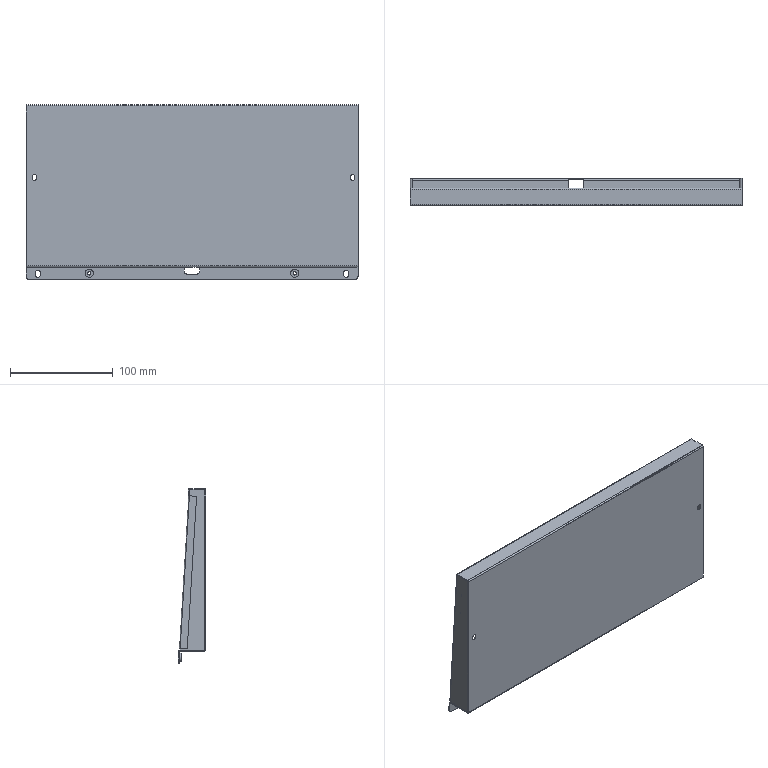Part | STEP file | TY.NE-0002-01-016A Keyboard tray-dddeger | 3 solids | 114 faces | box 323 x 27.127 x 169.984 mm | volume 77980 mm3 | plane 71 | cylinder 43 | commonest cylinder face diameters 0.6 x9 4 x6 5 x6 2.6 x5 3.3 x4 6 x4